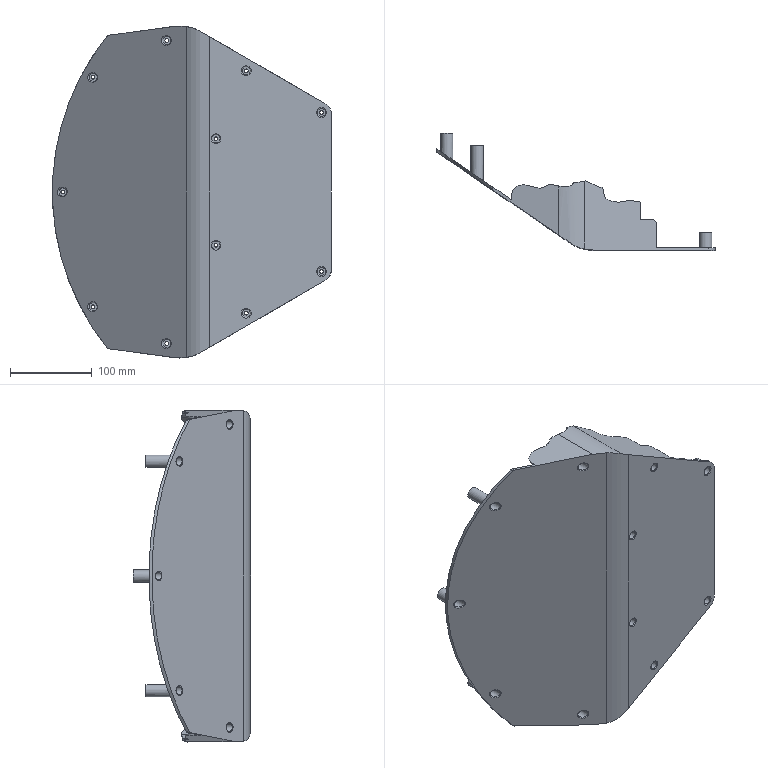Part | STEP file | NA609S-B | 1 solid | 222 faces | box 340.609 x 142.904 x 405.431 mm | volume 455741 mm3 | plane 90 | cylinder 66 | spline 60 | torus 6 | commonest cylinder face diameters 10 x13 4.5 x11 9 x11 15 x11 4 x10 6 x4